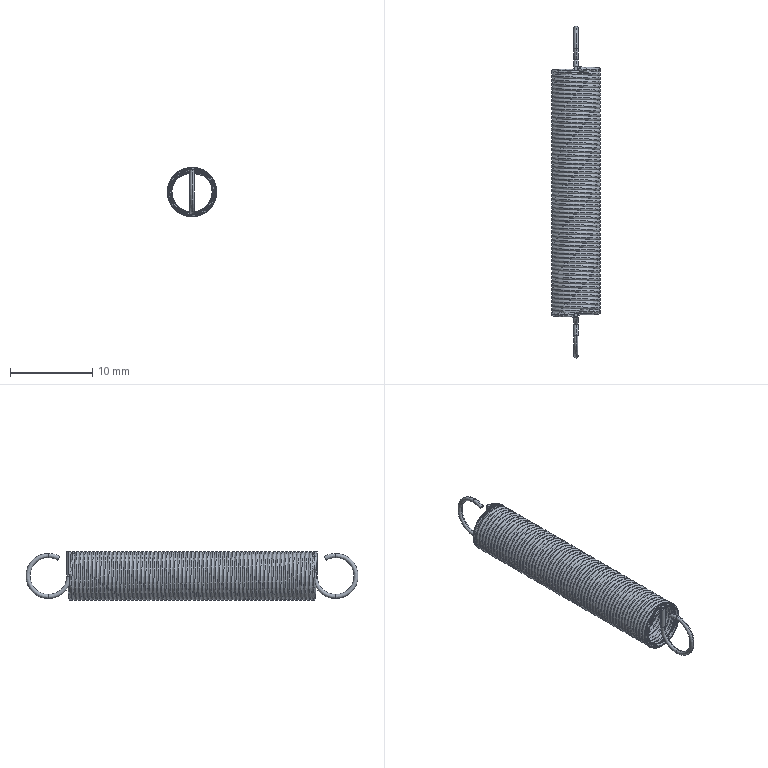Part | STEP file | 1 solid | 24 faces | box 6 x 40.5 x 6 mm | volume 206.632 mm3 | torus 12 | plane 4 | cylinder 4 | spline 4 | commonest cylinder face diameters 0.5 x4